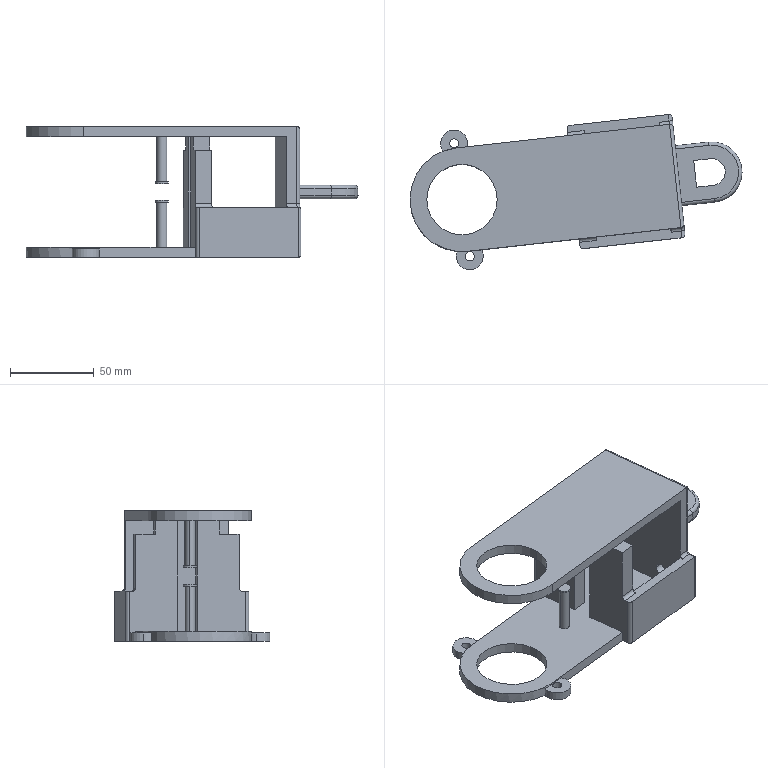Part | SolidWorks | features ICE 11, MirrorPattern 3, Fillet 2, Extrusion 1, HoleWzd 1, MirrorSolid 1 | 1 solid | 96 faces | box 198.087 x 92.564 x 78 mm | volume 194548 mm3 | cylinder 50 | plane 41 | torus 5 | commonest cylinder face diameters 4 x20 16 x7 6 x4 6.8 x4 8 x4 42 x4